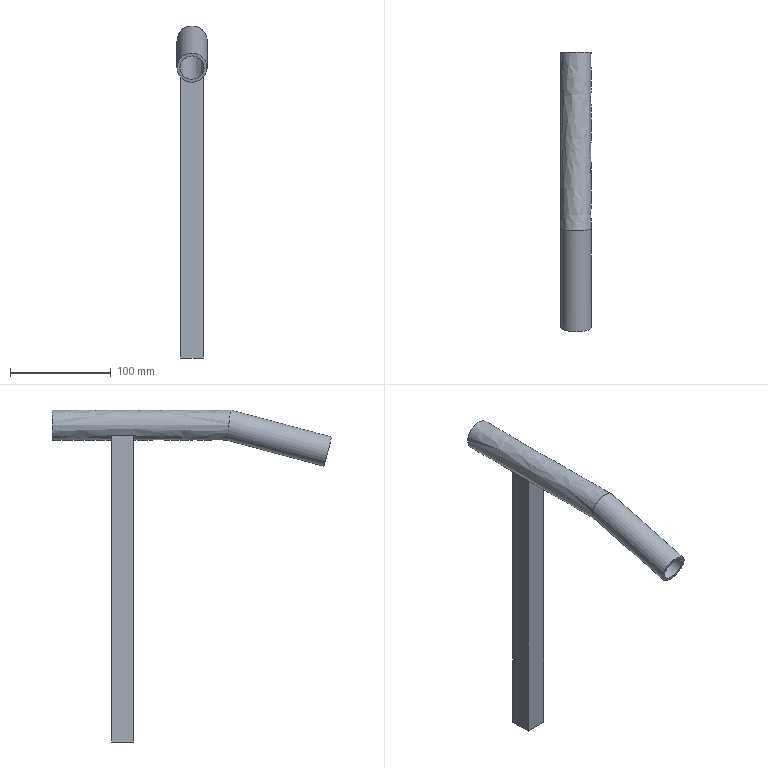Part | NX | features solid 2 | 1 solid | 22 faces | box 30 x 277.765 x 330 mm | volume 118575 mm3 | plane 15 | spline 7